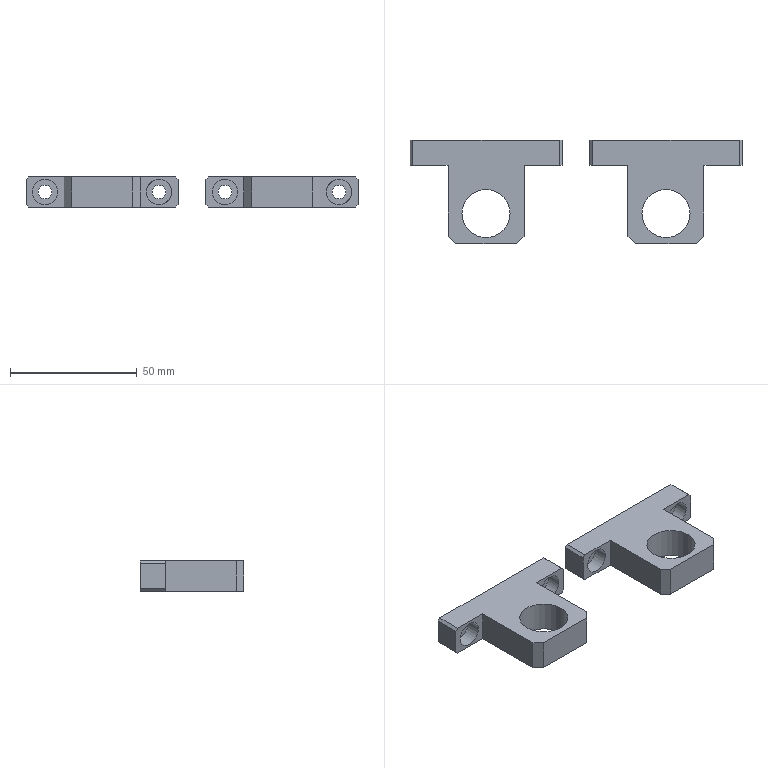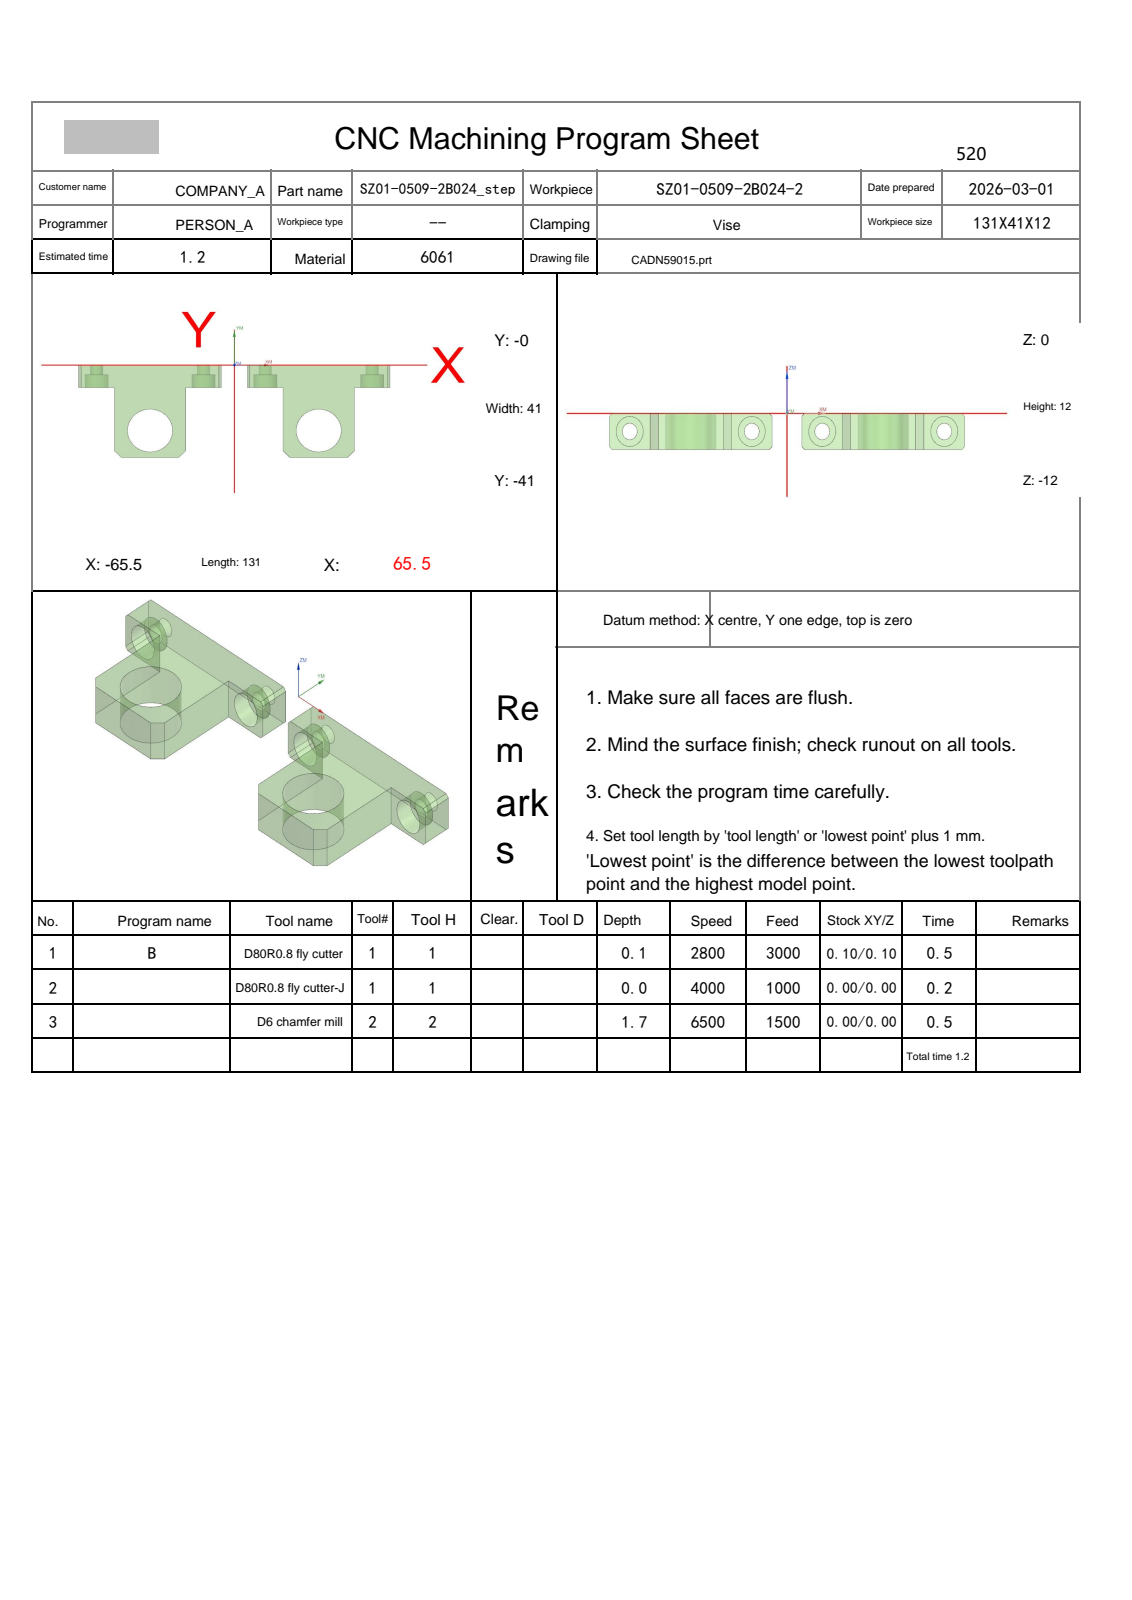NC program | NX | posted by the shop | part box 131 x 41 x 12 mm
Whole program:
%
O0001
(Machine time: 1.78 MIN)
(===Total Tool:2===)
(T1=D80R0.8 fly cutter D=80.  R=0.8  D-  H01 Z=0.    )
(T2=D6 chamfer mill   D=6.   R=0.   D-  H02 Z=-1.7  )
G80 G90 G17 G49 G40
G91 G28 Z0
M01
N1 T01 M06
(D80R0.8 fly cutter  D=80. R=0.8 H=01 ce=0.10 di=0.10)
G00 G90 G54 X-117.597 Y-20.5 M03 S2800
G43 H01 Z50.
M08
Z4.02
G01 Z2.02 F3000.
X-105.597
X105.597
X117.597
Z4.02
G00 X-117.597
Z3.54
G01 Z1.54
X-105.597
X105.597
X117.597
Z3.54
G00 X-117.597
Z3.06
G01 Z1.06
X-105.597
X105.597
X117.597
Z3.06
G00 X-117.597
Z2.58
G01 Z.58
X-105.597
X105.597
X117.597
Z2.58
G00 Z50.
X-117.597
Z2.1
G01 Z.1
X-105.597
X105.597
X117.597
Z2.1
G00 Z50.
G91 G28 Z0.0
M05
M09
G91 G28 Z0.0
M01
N2 T01 M06
(D80R0.8 fly cutter-J  D=80. R=0.8 H=01 ce=0.00 di=0.00)
G00 G90 G54 X-117.499 Y-20.5 M03 S4000
G43 H01 Z50.
M08
Z2.
G01 Z0.0 F1000.
X-105.499
X105.499
X117.499
Z2.
G00 Z50.
G91 G28 Z0.0
M05
M09
G91 G28 Z0.0
M01
N3 T02 M06
(D6 chamfer mill  D=6. R=0. H=02 ce=0.00 di=0.00)
G00 G90 G54 X-5.708 Y-10.99 M03 S6500
G43 H02 Z50.
M08
Z.13
G01 Z-1.2 F1500.
G03 X-6.048 Y-10.915 I-.601 J-1.907
G01 X-6.102 Y-10.905
X-6.151 Y-10.928
X-6.241 Y-10.966
X-6.5 Y-11.
X-19.5
Y-38.
X-19.534 Y-38.259
X-19.634 Y-38.5
X-19.793 Y-38.707
X-22.793 Y-41.707
X-23. Y-41.866
X-23.241 Y-41.966
X-23.5 Y-42.
X-47.5
X-47.759 Y-41.966
X-48. Y-41.866
X-48.207 Y-41.707
X-51.207 Y-38.707
X-51.366 Y-38.5
X-51.466 Y-38.259
X-51.5 Y-38.
Y-11.
X-64.5
X-64.759 Y-10.966
X-64.849 Y-10.928
X-64.898 Y-10.905
X-64.952 Y-10.915
G03 X-65.292 Y-10.99 I.261 J-1.983
G01 Z.13
G00 Z2.55
Y.99
Z.13
G01 Z-1.2
G03 X-64.952 Y.915 I.601 J1.907
G01 X-64.898 Y.905
X-64.849 Y.928
X-64.759 Y.966
X-64.5 Y1.
X-35.5
X-6.5
X-6.241 Y.966
X-6.151 Y.928
X-6.102 Y.905
X-6.048 Y.915
G03 X-5.708 Y.99 I-.261 J1.983
G01 Z.13
G00 Z10.
X-43.792 Y-28.604
Z.202
G01 Z-1.2
G03 X-43.978 Y-28.899 I1.592 J-1.211
G01 X-44.005 Y-28.946
X-44. Y-29.
G03 X-35.5 Y-37.5 I8.5 J0.0
X-27. Y-29. I0.0 J8.5
X-35.5 Y-20.5 I-8.5 J0.0
X-44. Y-29. I0.0 J-8.5
G01 X-44.005 Y-29.054
X-43.978 Y-29.101
G03 X-43.792 Y-29.396 I1.778 J.916
G01 Z.202
G00 Z10.
X65.292 Y-10.99
Z.13
G01 Z-1.2
G03 X64.952 Y-10.915 I-.601 J-1.907
G01 X64.898 Y-10.905
X64.849 Y-10.928
X64.759 Y-10.966
X64.5 Y-11.
X51.5
Y-38.
X51.466 Y-38.259
X51.366 Y-38.5
X51.207 Y-38.707
X48.207 Y-41.707
X48. Y-41.866
X47.759 Y-41.966
X47.5 Y-42.
X23.5
X23.241 Y-41.966
X23. Y-41.866
X22.793 Y-41.707
X19.793 Y-38.707
X19.634 Y-38.5
X19.534 Y-38.259
X19.5 Y-38.
Y-11.
X6.5
X6.241 Y-10.966
X6.151 Y-10.928
X6.102 Y-10.905
X6.048 Y-10.915
G03 X5.708 Y-10.99 I.261 J-1.983
G01 Z.13
G00 Z2.55
Y.99
Z.13
G01 Z-1.2
G03 X6.048 Y.915 I.601 J1.907
G01 X6.102 Y.905
X6.151 Y.928
X6.241 Y.966
X6.5 Y1.
X35.5
X64.5
X64.759 Y.966
X64.849 Y.928
X64.898 Y.905
X64.952 Y.915
G03 X65.292 Y.99 I-.261 J1.983
G01 Z.13
G00 Z10.
X27.208 Y-28.604
Z.202
G01 Z-1.2
G03 X27.022 Y-28.899 I1.592 J-1.211
G01 X26.995 Y-28.946
X27. Y-29.
G03 X35.5 Y-37.5 I8.5 J0.0
X44. Y-29. I0.0 J8.5
X35.5 Y-20.5 I-8.5 J0.0
X27. Y-29. I0.0 J-8.5
G01 X26.995 Y-29.054
X27.022 Y-29.101
G03 X27.208 Y-29.396 I1.778 J.916
G01 Z.202
G00 Z50.
G00 G90 X-66.208 Y-12.9 M03 S6500
Z50.
Z-.2
G01 Z-1.7 F1500.
X-66.199 Y-12.832
X-66.2 Y-12.763
Y2.763
X-66.199 Y2.832
X-66.208 Y2.9
Z-.2
G00 Z50.
X-4.792
Z-.2
G01 Z-1.7
X-4.801 Y2.832
X-4.8 Y2.763
Y-12.763
X-4.801 Y-12.832
X-4.792 Y-12.9
Z-.2
G00 X4.792
G01 Z-1.7
X4.801 Y-12.832
X4.8 Y-12.763
Y2.763
X4.801 Y2.832
X4.792 Y2.9
Z-.2
G00 Z50.
X66.208
Z-.2
G01 Z-1.7
X66.199 Y2.832
X66.2 Y2.763
Y-12.763
X66.199 Y-12.832
X66.208 Y-12.9
Z-.2
G00 Z50.
M05
M09
G91 G28 Z0.0
G91 G28 Y0.0
M30
%